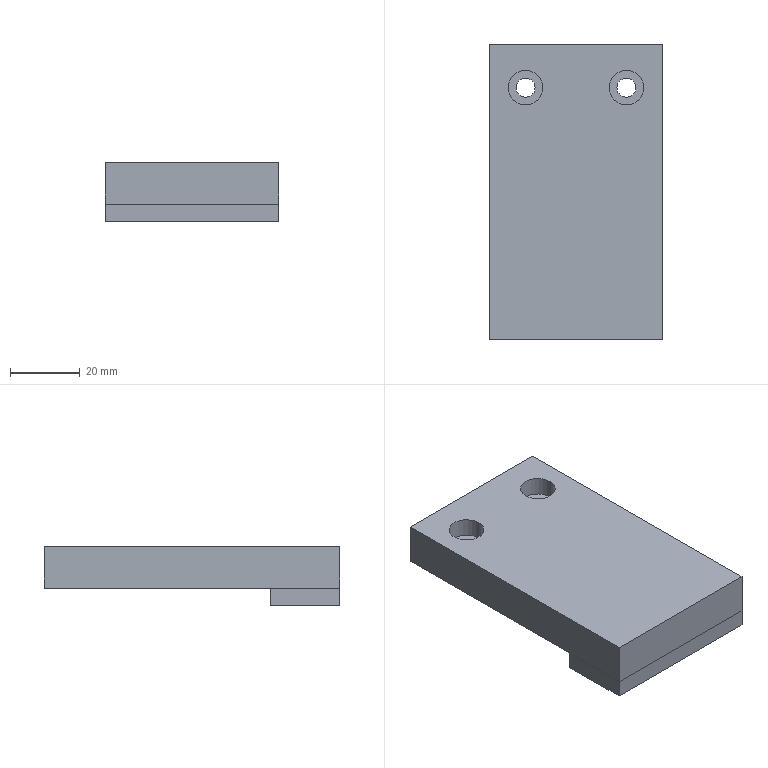Part | SolidWorks | features Extrusion 1, HoleWzd 1, ICE 1 | 2 solids | 22 faces | box 50 x 85 x 17 mm | volume 54838 mm3 | plane 14 | cylinder 8 | commonest cylinder face diameters 5.5 x4 10 x4
STEP:
#1=CARTESIAN_POINT('',(25.,-22.5,-6.));
#2=VERTEX_POINT('',#1);
#3=CARTESIAN_POINT('',(25.,-42.5,-6.));
#4=VERTEX_POINT('',#3);
#5=CARTESIAN_POINT('',(25.,-42.5,-6.));
#6=DIRECTION('',(0.,-1.,0.));
#7=VECTOR('',#6,1000.);
#8=LINE('',#5,#7);
#9=EDGE_CURVE('',#2,#4,#8,.T.);
#10=ORIENTED_EDGE('',*,*,#9,.T.);
#11=CARTESIAN_POINT('',(25.,-42.5,-11.));
#12=VERTEX_POINT('',#11);
#13=CARTESIAN_POINT('',(25.,-42.5,-11.));
#14=DIRECTION('',(0.,0.,1.));
#15=VECTOR('',#14,1000.);
#16=LINE('',#13,#15);
#17=EDGE_CURVE('',#12,#4,#16,.T.);
#18=ORIENTED_EDGE('',*,*,#17,.F.);
#19=CARTESIAN_POINT('',(25.,-22.5,-11.));
#20=VERTEX_POINT('',#19);
#21=CARTESIAN_POINT('',(25.,-42.5,-11.));
#22=DIRECTION('',(0.,-1.,0.));
#23=VECTOR('',#22,1000.);
#24=LINE('',#21,#23);
#25=EDGE_CURVE('',#20,#12,#24,.T.);
#26=ORIENTED_EDGE('',*,*,#25,.F.);
#27=CARTESIAN_POINT('',(25.,-22.5,-11.));
#28=DIRECTION('',(0.,0.,1.));
#29=VECTOR('',#28,1000.);
#30=LINE('',#27,#29);
#31=EDGE_CURVE('',#20,#2,#30,.T.);
#32=ORIENTED_EDGE('',*,*,#31,.T.);
#33=EDGE_LOOP('',(#10,#18,#26,#32));
#34=FACE_OUTER_BOUND('',#33,.T.);
#35=CARTESIAN_POINT('',(25.,-42.5,-11.));
#36=DIRECTION('',(-1.,0.,0.));
#37=DIRECTION('',(0.,0.,1.));
#38=AXIS2_PLACEMENT_3D('',#35,#36,#37);
#39=PLANE('',#38);
#40=ADVANCED_FACE('',(#34),#39,.F.);
#41=CARTESIAN_POINT('',(-25.,-42.5,-6.));
#42=VERTEX_POINT('',#41);
#43=CARTESIAN_POINT('',(25.,-42.5,-6.));
#44=DIRECTION('',(-1.,0.,0.));
#45=VECTOR('',#44,1000.);
#46=LINE('',#43,#45);
#47=EDGE_CURVE('',#4,#42,#46,.T.);
#48=ORIENTED_EDGE('',*,*,#47,.T.);
#49=CARTESIAN_POINT('',(-25.,-42.5,-11.));
#50=VERTEX_POINT('',#49);
#51=CARTESIAN_POINT('',(-25.,-42.5,-11.));
#52=DIRECTION('',(0.,0.,1.));
#53=VECTOR('',#52,1000.);
#54=LINE('',#51,#53);
#55=EDGE_CURVE('',#50,#42,#54,.T.);
#56=ORIENTED_EDGE('',*,*,#55,.F.);
#57=CARTESIAN_POINT('',(25.,-42.5,-11.));
#58=DIRECTION('',(-1.,0.,0.));
#59=VECTOR('',#58,1000.);
#60=LINE('',#57,#59);
#61=EDGE_CURVE('',#12,#50,#60,.T.);
#62=ORIENTED_EDGE('',*,*,#61,.F.);
#63=ORIENTED_EDGE('',*,*,#17,.T.);
#64=EDGE_LOOP('',(#48,#56,#62,#63));
#65=FACE_OUTER_BOUND('',#64,.T.);
#66=CARTESIAN_POINT('',(25.,-42.5,-11.));
#67=DIRECTION('',(0.,1.,0.));
#68=DIRECTION('',(0.,0.,1.));
#69=AXIS2_PLACEMENT_3D('',#66,#67,#68);
#70=PLANE('',#69);
#71=ADVANCED_FACE('',(#65),#70,.F.);
#72=CARTESIAN_POINT('',(-25.,-22.5,-6.));
#73=VERTEX_POINT('',#72);
#74=CARTESIAN_POINT('',(-25.,-42.5,-6.));
#75=DIRECTION('',(0.,1.,0.));
#76=VECTOR('',#75,1000.);
#77=LINE('',#74,#76);
#78=EDGE_CURVE('',#42,#73,#77,.T.);
#79=ORIENTED_EDGE('',*,*,#78,.T.);
#80=CARTESIAN_POINT('',(-25.,-22.5,-11.));
#81=VERTEX_POINT('',#80);
#82=CARTESIAN_POINT('',(-25.,-22.5,-11.));
#83=DIRECTION('',(0.,0.,1.));
#84=VECTOR('',#83,1000.);
#85=LINE('',#82,#84);
#86=EDGE_CURVE('',#81,#73,#85,.T.);
#87=ORIENTED_EDGE('',*,*,#86,.F.);
#88=CARTESIAN_POINT('',(-25.,-42.5,-11.));
#89=DIRECTION('',(0.,1.,0.));
#90=VECTOR('',#89,1000.);
#91=LINE('',#88,#90);
#92=EDGE_CURVE('',#50,#81,#91,.T.);
#93=ORIENTED_EDGE('',*,*,#92,.F.);
#94=ORIENTED_EDGE('',*,*,#55,.T.);
#95=EDGE_LOOP('',(#79,#87,#93,#94));
#96=FACE_OUTER_BOUND('',#95,.T.);
#97=CARTESIAN_POINT('',(-25.,-42.5,-11.));
#98=DIRECTION('',(1.,0.,0.));
#99=DIRECTION('',(0.,0.,-1.));
#100=AXIS2_PLACEMENT_3D('',#97,#98,#99);
#101=PLANE('',#100);
#102=ADVANCED_FACE('',(#96),#101,.F.);
#103=CARTESIAN_POINT('',(25.,-22.5,-6.));
#104=DIRECTION('',(1.,0.,0.));
#105=VECTOR('',#104,1000.);
#106=LINE('',#103,#105);
#107=EDGE_CURVE('',#73,#2,#106,.T.);
#108=ORIENTED_EDGE('',*,*,#107,.T.);
#109=ORIENTED_EDGE('',*,*,#31,.F.);
#110=CARTESIAN_POINT('',(25.,-22.5,-11.));
#111=DIRECTION('',(1.,0.,0.));
#112=VECTOR('',#111,1000.);
#113=LINE('',#110,#112);
#114=EDGE_CURVE('',#81,#20,#113,.T.);
#115=ORIENTED_EDGE('',*,*,#114,.F.);
#116=ORIENTED_EDGE('',*,*,#86,.T.);
#117=EDGE_LOOP('',(#108,#109,#115,#116));
#118=FACE_OUTER_BOUND('',#117,.T.);
#119=CARTESIAN_POINT('',(25.,-22.5,-11.));
#120=DIRECTION('',(0.,-1.,0.));
#121=DIRECTION('',(0.,0.,-1.));
#122=AXIS2_PLACEMENT_3D('',#119,#120,#121);
#123=PLANE('',#122);
#124=ADVANCED_FACE('',(#118),#123,.F.);
#125=ORIENTED_EDGE('',*,*,#25,.T.);
#126=ORIENTED_EDGE('',*,*,#61,.T.);
#127=ORIENTED_EDGE('',*,*,#92,.T.);
#128=ORIENTED_EDGE('',*,*,#114,.T.);
#129=EDGE_LOOP('',(#125,#126,#127,#128));
#130=FACE_OUTER_BOUND('',#129,.T.);
#131=CARTESIAN_POINT('',(0.,0.,-11.));
#132=DIRECTION('',(0.,0.,1.));
#133=DIRECTION('',(1.,0.,0.));
#134=AXIS2_PLACEMENT_3D('',#131,#132,#133);
#135=PLANE('',#134);
#136=ADVANCED_FACE('',(#130),#135,.F.);
#137=ORIENTED_EDGE('',*,*,#9,.F.);
#138=ORIENTED_EDGE('',*,*,#107,.F.);
#139=ORIENTED_EDGE('',*,*,#78,.F.);
#140=ORIENTED_EDGE('',*,*,#47,.F.);
#141=EDGE_LOOP('',(#137,#138,#139,#140));
#142=FACE_OUTER_BOUND('',#141,.T.);
#143=CARTESIAN_POINT('',(0.,0.,-6.));
#144=DIRECTION('',(0.,0.,1.));
#145=DIRECTION('',(1.,0.,0.));
#146=AXIS2_PLACEMENT_3D('',#143,#144,#145);
#147=PLANE('',#146);
#148=ADVANCED_FACE('',(#142),#147,.T.);
#149=CLOSED_SHELL('',(#40,#71,#102,#124,#136,#148));
#150=MANIFOLD_SOLID_BREP('',#149);
#151=CARTESIAN_POINT('',(-19.5,30.,0.6));
#152=VERTEX_POINT('',#151);
#153=CARTESIAN_POINT('',(-9.5,30.,0.6));
#154=VERTEX_POINT('',#153);
#155=CARTESIAN_POINT('',(-14.5,30.,0.6));
#156=DIRECTION('',(0.,0.,1.));
#157=DIRECTION('',(1.,0.,0.));
#158=AXIS2_PLACEMENT_3D('',#155,#156,#157);
#159=CIRCLE('',#158,5.);
#160=EDGE_CURVE('',#152,#154,#159,.T.);
#161=ORIENTED_EDGE('',*,*,#160,.F.);
#162=CARTESIAN_POINT('',(-19.5,30.,6.));
#163=VERTEX_POINT('',#162);
#164=CARTESIAN_POINT('',(-19.5,30.,6.));
#165=DIRECTION('',(0.,0.,1.));
#166=VECTOR('',#165,1000.);
#167=LINE('',#164,#166);
#168=EDGE_CURVE('',#152,#163,#167,.T.);
#169=ORIENTED_EDGE('',*,*,#168,.T.);
#170=CARTESIAN_POINT('',(-9.5,30.,6.));
#171=VERTEX_POINT('',#170);
#172=CARTESIAN_POINT('',(-14.5,30.,6.));
#173=DIRECTION('',(0.,0.,1.));
#174=DIRECTION('',(1.,0.,0.));
#175=AXIS2_PLACEMENT_3D('',#172,#173,#174);
#176=CIRCLE('',#175,5.);
#177=EDGE_CURVE('',#163,#171,#176,.T.);
#178=ORIENTED_EDGE('',*,*,#177,.T.);
#179=CARTESIAN_POINT('',(-9.5,30.,6.));
#180=DIRECTION('',(0.,0.,1.));
#181=VECTOR('',#180,1000.);
#182=LINE('',#179,#181);
#183=EDGE_CURVE('',#154,#171,#182,.T.);
#184=ORIENTED_EDGE('',*,*,#183,.F.);
#185=EDGE_LOOP('',(#161,#169,#178,#184));
#186=FACE_OUTER_BOUND('',#185,.T.);
#187=CARTESIAN_POINT('',(-14.5,30.,6.));
#188=DIRECTION('',(0.,0.,1.));
#189=DIRECTION('',(1.,0.,0.));
#190=AXIS2_PLACEMENT_3D('',#187,#188,#189);
#191=CYLINDRICAL_SURFACE('',#190,5.);
#192=ADVANCED_FACE('',(#186),#191,.F.);
#193=CARTESIAN_POINT('',(-11.75,30.,-6.));
#194=VERTEX_POINT('',#193);
#195=CARTESIAN_POINT('',(-17.25,30.,-6.));
#196=VERTEX_POINT('',#195);
#197=CARTESIAN_POINT('',(-14.5,30.,-6.));
#198=DIRECTION('',(0.,0.,-1.));
#199=DIRECTION('',(-1.,0.,0.));
#200=AXIS2_PLACEMENT_3D('',#197,#198,#199);
#201=CIRCLE('',#200,2.75);
#202=EDGE_CURVE('',#194,#196,#201,.T.);
#203=ORIENTED_EDGE('',*,*,#202,.T.);
#204=CARTESIAN_POINT('',(-17.25,30.,0.6));
#205=VERTEX_POINT('',#204);
#206=CARTESIAN_POINT('',(-17.25,30.,6.));
#207=DIRECTION('',(0.,0.,1.));
#208=VECTOR('',#207,1000.);
#209=LINE('',#206,#208);
#210=EDGE_CURVE('',#196,#205,#209,.T.);
#211=ORIENTED_EDGE('',*,*,#210,.T.);
#212=CARTESIAN_POINT('',(-11.75,30.,0.6));
#213=VERTEX_POINT('',#212);
#214=CARTESIAN_POINT('',(-14.5,30.,0.6));
#215=DIRECTION('',(0.,0.,1.));
#216=DIRECTION('',(1.,0.,0.));
#217=AXIS2_PLACEMENT_3D('',#214,#215,#216);
#218=CIRCLE('',#217,2.75);
#219=EDGE_CURVE('',#205,#213,#218,.T.);
#220=ORIENTED_EDGE('',*,*,#219,.T.);
#221=CARTESIAN_POINT('',(-11.75,30.,6.));
#222=DIRECTION('',(0.,0.,1.));
#223=VECTOR('',#222,1000.);
#224=LINE('',#221,#223);
#225=EDGE_CURVE('',#194,#213,#224,.T.);
#226=ORIENTED_EDGE('',*,*,#225,.F.);
#227=EDGE_LOOP('',(#203,#211,#220,#226));
#228=FACE_OUTER_BOUND('',#227,.T.);
#229=CARTESIAN_POINT('',(-14.5,30.,6.));
#230=DIRECTION('',(0.,0.,1.));
#231=DIRECTION('',(1.,0.,0.));
#232=AXIS2_PLACEMENT_3D('',#229,#230,#231);
#233=CYLINDRICAL_SURFACE('',#232,2.75);
#234=ADVANCED_FACE('',(#228),#233,.F.);
#235=CARTESIAN_POINT('',(9.5,30.,0.6));
#236=VERTEX_POINT('',#235);
#237=CARTESIAN_POINT('',(19.5,30.,0.6));
#238=VERTEX_POINT('',#237);
#239=CARTESIAN_POINT('',(14.5,30.,0.6));
#240=DIRECTION('',(0.,0.,1.));
#241=DIRECTION('',(1.,0.,0.));
#242=AXIS2_PLACEMENT_3D('',#239,#240,#241);
#243=CIRCLE('',#242,5.);
#244=EDGE_CURVE('',#236,#238,#243,.T.);
#245=ORIENTED_EDGE('',*,*,#244,.F.);
#246=CARTESIAN_POINT('',(9.5,30.,6.));
#247=VERTEX_POINT('',#246);
#248=CARTESIAN_POINT('',(9.5,30.,6.));
#249=DIRECTION('',(0.,0.,1.));
#250=VECTOR('',#249,1000.);
#251=LINE('',#248,#250);
#252=EDGE_CURVE('',#236,#247,#251,.T.);
#253=ORIENTED_EDGE('',*,*,#252,.T.);
#254=CARTESIAN_POINT('',(19.5,30.,6.));
#255=VERTEX_POINT('',#254);
#256=CARTESIAN_POINT('',(14.5,30.,6.));
#257=DIRECTION('',(0.,0.,1.));
#258=DIRECTION('',(1.,0.,0.));
#259=AXIS2_PLACEMENT_3D('',#256,#257,#258);
#260=CIRCLE('',#259,5.);
#261=EDGE_CURVE('',#247,#255,#260,.T.);
#262=ORIENTED_EDGE('',*,*,#261,.T.);
#263=CARTESIAN_POINT('',(19.5,30.,6.));
#264=DIRECTION('',(0.,0.,1.));
#265=VECTOR('',#264,1000.);
#266=LINE('',#263,#265);
#267=EDGE_CURVE('',#238,#255,#266,.T.);
#268=ORIENTED_EDGE('',*,*,#267,.F.);
#269=EDGE_LOOP('',(#245,#253,#262,#268));
#270=FACE_OUTER_BOUND('',#269,.T.);
#271=CARTESIAN_POINT('',(14.5,30.,6.));
#272=DIRECTION('',(0.,0.,1.));
#273=DIRECTION('',(1.,0.,0.));
#274=AXIS2_PLACEMENT_3D('',#271,#272,#273);
#275=CYLINDRICAL_SURFACE('',#274,5.);
#276=ADVANCED_FACE('',(#270),#275,.F.);
#277=CARTESIAN_POINT('',(17.25,30.,-6.));
#278=VERTEX_POINT('',#277);
#279=CARTESIAN_POINT('',(11.75,30.,-6.));
#280=VERTEX_POINT('',#279);
#281=CARTESIAN_POINT('',(14.5,30.,-6.));
#282=DIRECTION('',(0.,0.,-1.));
#283=DIRECTION('',(-1.,0.,0.));
#284=AXIS2_PLACEMENT_3D('',#281,#282,#283);
#285=CIRCLE('',#284,2.75);
#286=EDGE_CURVE('',#278,#280,#285,.T.);
#287=ORIENTED_EDGE('',*,*,#286,.T.);
#288=CARTESIAN_POINT('',(11.75,30.,0.6));
#289=VERTEX_POINT('',#288);
#290=CARTESIAN_POINT('',(11.75,30.,6.));
#291=DIRECTION('',(0.,0.,1.));
#292=VECTOR('',#291,1000.);
#293=LINE('',#290,#292);
#294=EDGE_CURVE('',#280,#289,#293,.T.);
#295=ORIENTED_EDGE('',*,*,#294,.T.);
#296=CARTESIAN_POINT('',(17.25,30.,0.6));
#297=VERTEX_POINT('',#296);
#298=CARTESIAN_POINT('',(14.5,30.,0.6));
#299=DIRECTION('',(0.,0.,1.));
#300=DIRECTION('',(1.,0.,0.));
#301=AXIS2_PLACEMENT_3D('',#298,#299,#300);
#302=CIRCLE('',#301,2.75);
#303=EDGE_CURVE('',#289,#297,#302,.T.);
#304=ORIENTED_EDGE('',*,*,#303,.T.);
#305=CARTESIAN_POINT('',(17.25,30.,6.));
#306=DIRECTION('',(0.,0.,1.));
#307=VECTOR('',#306,1000.);
#308=LINE('',#305,#307);
#309=EDGE_CURVE('',#278,#297,#308,.T.);
#310=ORIENTED_EDGE('',*,*,#309,.F.);
#311=EDGE_LOOP('',(#287,#295,#304,#310));
#312=FACE_OUTER_BOUND('',#311,.T.);
#313=CARTESIAN_POINT('',(14.5,30.,6.));
#314=DIRECTION('',(0.,0.,1.));
#315=DIRECTION('',(1.,0.,0.));
#316=AXIS2_PLACEMENT_3D('',#313,#314,#315);
#317=CYLINDRICAL_SURFACE('',#316,2.75);
#318=ADVANCED_FACE('',(#312),#317,.F.);
#319=CARTESIAN_POINT('',(25.,-42.5,-6.));
#320=VERTEX_POINT('',#319);
#321=CARTESIAN_POINT('',(25.,42.5,-6.));
#322=VERTEX_POINT('',#321);
#323=CARTESIAN_POINT('',(25.,-42.5,-6.));
#324=DIRECTION('',(0.,1.,0.));
#325=VECTOR('',#324,1000.);
#326=LINE('',#323,#325);
#327=EDGE_CURVE('',#320,#322,#326,.T.);
#328=ORIENTED_EDGE('',*,*,#327,.T.);
#329=CARTESIAN_POINT('',(25.,42.5,6.));
#330=VERTEX_POINT('',#329);
#331=CARTESIAN_POINT('',(25.,42.5,6.));
#332=DIRECTION('',(0.,0.,-1.));
#333=VECTOR('',#332,1000.);
#334=LINE('',#331,#333);
#335=EDGE_CURVE('',#330,#322,#334,.T.);
#336=ORIENTED_EDGE('',*,*,#335,.F.);
#337=CARTESIAN_POINT('',(25.,-42.5,6.));
#338=VERTEX_POINT('',#337);
#339=CARTESIAN_POINT('',(25.,-42.5,6.));
#340=DIRECTION('',(0.,1.,0.));
#341=VECTOR('',#340,1000.);
#342=LINE('',#339,#341);
#343=EDGE_CURVE('',#338,#330,#342,.T.);
#344=ORIENTED_EDGE('',*,*,#343,.F.);
#345=CARTESIAN_POINT('',(25.,-42.5,6.));
#346=DIRECTION('',(0.,0.,-1.));
#347=VECTOR('',#346,1000.);
#348=LINE('',#345,#347);
#349=EDGE_CURVE('',#338,#320,#348,.T.);
#350=ORIENTED_EDGE('',*,*,#349,.T.);
#351=EDGE_LOOP('',(#328,#336,#344,#350));
#352=FACE_OUTER_BOUND('',#351,.T.);
#353=CARTESIAN_POINT('',(25.,-42.5,6.));
#354=DIRECTION('',(-1.,0.,0.));
#355=DIRECTION('',(0.,0.,1.));
#356=AXIS2_PLACEMENT_3D('',#353,#354,#355);
#357=PLANE('',#356);
#358=ADVANCED_FACE('',(#352),#357,.F.);
#359=CARTESIAN_POINT('',(-25.,42.5,-6.));
#360=VERTEX_POINT('',#359);
#361=CARTESIAN_POINT('',(-25.,42.5,-6.));
#362=DIRECTION('',(-1.,0.,0.));
#363=VECTOR('',#362,1000.);
#364=LINE('',#361,#363);
#365=EDGE_CURVE('',#322,#360,#364,.T.);
#366=ORIENTED_EDGE('',*,*,#365,.T.);
#367=CARTESIAN_POINT('',(-25.,42.5,6.));
#368=VERTEX_POINT('',#367);
#369=CARTESIAN_POINT('',(-25.,42.5,6.));
#370=DIRECTION('',(0.,0.,-1.));
#371=VECTOR('',#370,1000.);
#372=LINE('',#369,#371);
#373=EDGE_CURVE('',#368,#360,#372,.T.);
#374=ORIENTED_EDGE('',*,*,#373,.F.);
#375=CARTESIAN_POINT('',(-25.,42.5,6.));
#376=DIRECTION('',(-1.,0.,0.));
#377=VECTOR('',#376,1000.);
#378=LINE('',#375,#377);
#379=EDGE_CURVE('',#330,#368,#378,.T.);
#380=ORIENTED_EDGE('',*,*,#379,.F.);
#381=ORIENTED_EDGE('',*,*,#335,.T.);
#382=EDGE_LOOP('',(#366,#374,#380,#381));
#383=FACE_OUTER_BOUND('',#382,.T.);
#384=CARTESIAN_POINT('',(-25.,42.5,6.));
#385=DIRECTION('',(0.,-1.,0.));
#386=DIRECTION('',(0.,0.,-1.));
#387=AXIS2_PLACEMENT_3D('',#384,#385,#386);
#388=PLANE('',#387);
#389=ADVANCED_FACE('',(#383),#388,.F.);
#390=CARTESIAN_POINT('',(-25.,-42.5,-6.));
#391=VERTEX_POINT('',#390);
#392=CARTESIAN_POINT('',(-25.,-42.5,-6.));
#393=DIRECTION('',(0.,-1.,0.));
#394=VECTOR('',#393,1000.);
#395=LINE('',#392,#394);
#396=EDGE_CURVE('',#360,#391,#395,.T.);
#397=ORIENTED_EDGE('',*,*,#396,.T.);
#398=CARTESIAN_POINT('',(-25.,-42.5,6.));
#399=VERTEX_POINT('',#398);
#400=CARTESIAN_POINT('',(-25.,-42.5,6.));
#401=DIRECTION('',(0.,0.,-1.));
#402=VECTOR('',#401,1000.);
#403=LINE('',#400,#402);
#404=EDGE_CURVE('',#399,#391,#403,.T.);
#405=ORIENTED_EDGE('',*,*,#404,.F.);
#406=CARTESIAN_POINT('',(-25.,-42.5,6.));
#407=DIRECTION('',(0.,-1.,0.));
#408=VECTOR('',#407,1000.);
#409=LINE('',#406,#408);
#410=EDGE_CURVE('',#368,#399,#409,.T.);
#411=ORIENTED_EDGE('',*,*,#410,.F.);
#412=ORIENTED_EDGE('',*,*,#373,.T.);
#413=EDGE_LOOP('',(#397,#405,#411,#412));
#414=FACE_OUTER_BOUND('',#413,.T.);
#415=CARTESIAN_POINT('',(-25.,-42.5,6.));
#416=DIRECTION('',(1.,0.,0.));
#417=DIRECTION('',(0.,0.,-1.));
#418=AXIS2_PLACEMENT_3D('',#415,#416,#417);
#419=PLANE('',#418);
#420=ADVANCED_FACE('',(#414),#419,.F.);
#421=CARTESIAN_POINT('',(-25.,-42.5,-6.));
#422=DIRECTION('',(1.,0.,0.));
#423=VECTOR('',#422,1000.);
#424=LINE('',#421,#423);
#425=EDGE_CURVE('',#391,#320,#424,.T.);
#426=ORIENTED_EDGE('',*,*,#425,.T.);
#427=ORIENTED_EDGE('',*,*,#349,.F.);
#428=CARTESIAN_POINT('',(-25.,-42.5,6.));
#429=DIRECTION('',(1.,0.,0.));
#430=VECTOR('',#429,1000.);
#431=LINE('',#428,#430);
#432=EDGE_CURVE('',#399,#338,#431,.T.);
#433=ORIENTED_EDGE('',*,*,#432,.F.);
#434=ORIENTED_EDGE('',*,*,#404,.T.);
#435=EDGE_LOOP('',(#426,#427,#433,#434));
#436=FACE_OUTER_BOUND('',#435,.T.);
#437=CARTESIAN_POINT('',(-25.,-42.5,6.));
#438=DIRECTION('',(0.,1.,0.));
#439=DIRECTION('',(0.,0.,1.));
#440=AXIS2_PLACEMENT_3D('',#437,#438,#439);
#441=PLANE('',#440);
#442=ADVANCED_FACE('',(#436),#441,.F.);
#443=CARTESIAN_POINT('',(-14.5,30.,6.));
#444=DIRECTION('',(0.,0.,1.));
#445=DIRECTION('',(1.,0.,0.));
#446=AXIS2_PLACEMENT_3D('',#443,#444,#445);
#447=CIRCLE('',#446,5.);
#448=EDGE_CURVE('',#171,#163,#447,.T.);
#449=ORIENTED_EDGE('',*,*,#448,.F.);
#450=ORIENTED_EDGE('',*,*,#177,.F.);
#451=EDGE_LOOP('',(#449,#450));
#452=FACE_BOUND('',#451,.T.);
#453=CARTESIAN_POINT('',(14.5,30.,6.));
#454=DIRECTION('',(0.,0.,1.));
#455=DIRECTION('',(1.,0.,0.));
#456=AXIS2_PLACEMENT_3D('',#453,#454,#455);
#457=CIRCLE('',#456,5.);
#458=EDGE_CURVE('',#255,#247,#457,.T.);
#459=ORIENTED_EDGE('',*,*,#458,.F.);
#460=ORIENTED_EDGE('',*,*,#261,.F.);
#461=EDGE_LOOP('',(#459,#460));
#462=FACE_BOUND('',#461,.T.);
#463=ORIENTED_EDGE('',*,*,#343,.T.);
#464=ORIENTED_EDGE('',*,*,#379,.T.);
#465=ORIENTED_EDGE('',*,*,#410,.T.);
#466=ORIENTED_EDGE('',*,*,#432,.T.);
#467=EDGE_LOOP('',(#463,#464,#465,#466));
#468=FACE_OUTER_BOUND('',#467,.T.);
#469=CARTESIAN_POINT('',(0.,0.,6.));
#470=DIRECTION('',(0.,0.,-1.));
#471=DIRECTION('',(-1.,0.,0.));
#472=AXIS2_PLACEMENT_3D('',#469,#470,#471);
#473=PLANE('',#472);
#474=ADVANCED_FACE('',(#452,#462,#468),#473,.F.);
#475=ORIENTED_EDGE('',*,*,#202,.F.);
#476=CARTESIAN_POINT('',(-14.5,30.,-6.));
#477=DIRECTION('',(0.,0.,-1.));
#478=DIRECTION('',(-1.,0.,0.));
#479=AXIS2_PLACEMENT_3D('',#476,#477,#478);
#480=CIRCLE('',#479,2.75);
#481=EDGE_CURVE('',#196,#194,#480,.T.);
#482=ORIENTED_EDGE('',*,*,#481,.F.);
#483=EDGE_LOOP('',(#475,#482));
#484=FACE_BOUND('',#483,.T.);
#485=ORIENTED_EDGE('',*,*,#286,.F.);
#486=CARTESIAN_POINT('',(14.5,30.,-6.));
#487=DIRECTION('',(0.,0.,-1.));
#488=DIRECTION('',(-1.,0.,0.));
#489=AXIS2_PLACEMENT_3D('',#486,#487,#488);
#490=CIRCLE('',#489,2.75);
#491=EDGE_CURVE('',#280,#278,#490,.T.);
#492=ORIENTED_EDGE('',*,*,#491,.F.);
#493=EDGE_LOOP('',(#485,#492));
#494=FACE_BOUND('',#493,.T.);
#495=ORIENTED_EDGE('',*,*,#327,.F.);
#496=ORIENTED_EDGE('',*,*,#425,.F.);
#497=ORIENTED_EDGE('',*,*,#396,.F.);
#498=ORIENTED_EDGE('',*,*,#365,.F.);
#499=EDGE_LOOP('',(#495,#496,#497,#498));
#500=FACE_OUTER_BOUND('',#499,.T.);
#501=CARTESIAN_POINT('',(0.,0.,-6.));
#502=DIRECTION('',(0.,0.,-1.));
#503=DIRECTION('',(-1.,0.,0.));
#504=AXIS2_PLACEMENT_3D('',#501,#502,#503);
#505=PLANE('',#504);
#506=ADVANCED_FACE('',(#484,#494,#500),#505,.T.);
#507=ORIENTED_EDGE('',*,*,#294,.F.);
#508=ORIENTED_EDGE('',*,*,#491,.T.);
#509=ORIENTED_EDGE('',*,*,#309,.T.);
#510=CARTESIAN_POINT('',(14.5,30.,0.6));
#511=DIRECTION('',(0.,0.,1.));
#512=DIRECTION('',(1.,0.,0.));
#513=AXIS2_PLACEMENT_3D('',#510,#511,#512);
#514=CIRCLE('',#513,2.75);
#515=EDGE_CURVE('',#297,#289,#514,.T.);
#516=ORIENTED_EDGE('',*,*,#515,.T.);
#517=EDGE_LOOP('',(#507,#508,#509,#516));
#518=FACE_OUTER_BOUND('',#517,.T.);
#519=CARTESIAN_POINT('',(14.5,30.,6.));
#520=DIRECTION('',(0.,0.,1.));
#521=DIRECTION('',(1.,0.,0.));
#522=AXIS2_PLACEMENT_3D('',#519,#520,#521);
#523=CYLINDRICAL_SURFACE('',#522,2.75);
#524=ADVANCED_FACE('',(#518),#523,.F.);
#525=ORIENTED_EDGE('',*,*,#515,.F.);
#526=ORIENTED_EDGE('',*,*,#303,.F.);
#527=EDGE_LOOP('',(#525,#526));
#528=FACE_BOUND('',#527,.T.);
#529=CARTESIAN_POINT('',(14.5,30.,0.6));
#530=DIRECTION('',(0.,0.,1.));
#531=DIRECTION('',(1.,0.,0.));
#532=AXIS2_PLACEMENT_3D('',#529,#530,#531);
#533=CIRCLE('',#532,5.);
#534=EDGE_CURVE('',#238,#236,#533,.T.);
#535=ORIENTED_EDGE('',*,*,#534,.T.);
#536=ORIENTED_EDGE('',*,*,#244,.T.);
#537=EDGE_LOOP('',(#535,#536));
#538=FACE_OUTER_BOUND('',#537,.T.);
#539=CARTESIAN_POINT('',(17.25,30.,0.6));
#540=DIRECTION('',(0.,0.,-1.));
#541=DIRECTION('',(-1.,0.,0.));
#542=AXIS2_PLACEMENT_3D('',#539,#540,#541);
#543=PLANE('',#542);
#544=ADVANCED_FACE('',(#528,#538),#543,.F.);
#545=ORIENTED_EDGE('',*,*,#252,.F.);
#546=ORIENTED_EDGE('',*,*,#534,.F.);
#547=ORIENTED_EDGE('',*,*,#267,.T.);
#548=ORIENTED_EDGE('',*,*,#458,.T.);
#549=EDGE_LOOP('',(#545,#546,#547,#548));
#550=FACE_OUTER_BOUND('',#549,.T.);
#551=CARTESIAN_POINT('',(14.5,30.,6.));
#552=DIRECTION('',(0.,0.,1.));
#553=DIRECTION('',(1.,0.,0.));
#554=AXIS2_PLACEMENT_3D('',#551,#552,#553);
#555=CYLINDRICAL_SURFACE('',#554,5.);
#556=ADVANCED_FACE('',(#550),#555,.F.);
#557=ORIENTED_EDGE('',*,*,#210,.F.);
#558=ORIENTED_EDGE('',*,*,#481,.T.);
#559=ORIENTED_EDGE('',*,*,#225,.T.);
#560=CARTESIAN_POINT('',(-14.5,30.,0.6));
#561=DIRECTION('',(0.,0.,1.));
#562=DIRECTION('',(1.,0.,0.));
#563=AXIS2_PLACEMENT_3D('',#560,#561,#562);
#564=CIRCLE('',#563,2.75);
#565=EDGE_CURVE('',#213,#205,#564,.T.);
#566=ORIENTED_EDGE('',*,*,#565,.T.);
#567=EDGE_LOOP('',(#557,#558,#559,#566));
#568=FACE_OUTER_BOUND('',#567,.T.);
#569=CARTESIAN_POINT('',(-14.5,30.,6.));
#570=DIRECTION('',(0.,0.,1.));
#571=DIRECTION('',(1.,0.,0.));
#572=AXIS2_PLACEMENT_3D('',#569,#570,#571);
#573=CYLINDRICAL_SURFACE('',#572,2.75);
#574=ADVANCED_FACE('',(#568),#573,.F.);
#575=ORIENTED_EDGE('',*,*,#565,.F.);
#576=ORIENTED_EDGE('',*,*,#219,.F.);
#577=EDGE_LOOP('',(#575,#576));
#578=FACE_BOUND('',#577,.T.);
#579=CARTESIAN_POINT('',(-14.5,30.,0.6));
#580=DIRECTION('',(0.,0.,1.));
#581=DIRECTION('',(1.,0.,0.));
#582=AXIS2_PLACEMENT_3D('',#579,#580,#581);
#583=CIRCLE('',#582,5.);
#584=EDGE_CURVE('',#154,#152,#583,.T.);
#585=ORIENTED_EDGE('',*,*,#584,.T.);
#586=ORIENTED_EDGE('',*,*,#160,.T.);
#587=EDGE_LOOP('',(#585,#586));
#588=FACE_OUTER_BOUND('',#587,.T.);
#589=CARTESIAN_POINT('',(-11.75,30.,0.6));
#590=DIRECTION('',(0.,0.,-1.));
#591=DIRECTION('',(-1.,0.,0.));
#592=AXIS2_PLACEMENT_3D('',#589,#590,#591);
#593=PLANE('',#592);
#594=ADVANCED_FACE('',(#578,#588),#593,.F.);
#595=ORIENTED_EDGE('',*,*,#168,.F.);
#596=ORIENTED_EDGE('',*,*,#584,.F.);
#597=ORIENTED_EDGE('',*,*,#183,.T.);
#598=ORIENTED_EDGE('',*,*,#448,.T.);
#599=EDGE_LOOP('',(#595,#596,#597,#598));
#600=FACE_OUTER_BOUND('',#599,.T.);
#601=CARTESIAN_POINT('',(-14.5,30.,6.));
#602=DIRECTION('',(0.,0.,1.));
#603=DIRECTION('',(1.,0.,0.));
#604=AXIS2_PLACEMENT_3D('',#601,#602,#603);
#605=CYLINDRICAL_SURFACE('',#604,5.);
#606=ADVANCED_FACE('',(#600),#605,.F.);
#607=CLOSED_SHELL('',(#192,#234,#276,#318,#358,#389,#420,#442,#474,#506,#524,#544,#556,#574,#594,#606));
#608=MANIFOLD_SOLID_BREP('',#607);
#609=CARTESIAN_POINT('',(0.,0.,0.));
#610=DIRECTION('',(0.,0.,1.));
#611=DIRECTION('',(1.,0.,0.));
#612=AXIS2_PLACEMENT_3D('',#609,#610,#611);
#613=(LENGTH_UNIT()NAMED_UNIT(*)SI_UNIT(.MILLI.,.METRE.));
#614=UNCERTAINTY_MEASURE_WITH_UNIT(LENGTH_MEASURE(0.00001),#613,'','');
#615=(NAMED_UNIT(*)PLANE_ANGLE_UNIT()SI_UNIT($,.RADIAN.));
#616=(NAMED_UNIT(*)SI_UNIT($,.STERADIAN.)SOLID_ANGLE_UNIT());
#617=(GEOMETRIC_REPRESENTATION_CONTEXT(3)GLOBAL_UNCERTAINTY_ASSIGNED_CONTEXT((#614))GLOBAL_UNIT_ASSIGNED_CONTEXT((#613,#615,#616))REPRESENTATION_CONTEXT('',''));
#618=ADVANCED_BREP_SHAPE_REPRESENTATION('',(#150,#608,#612),#617);